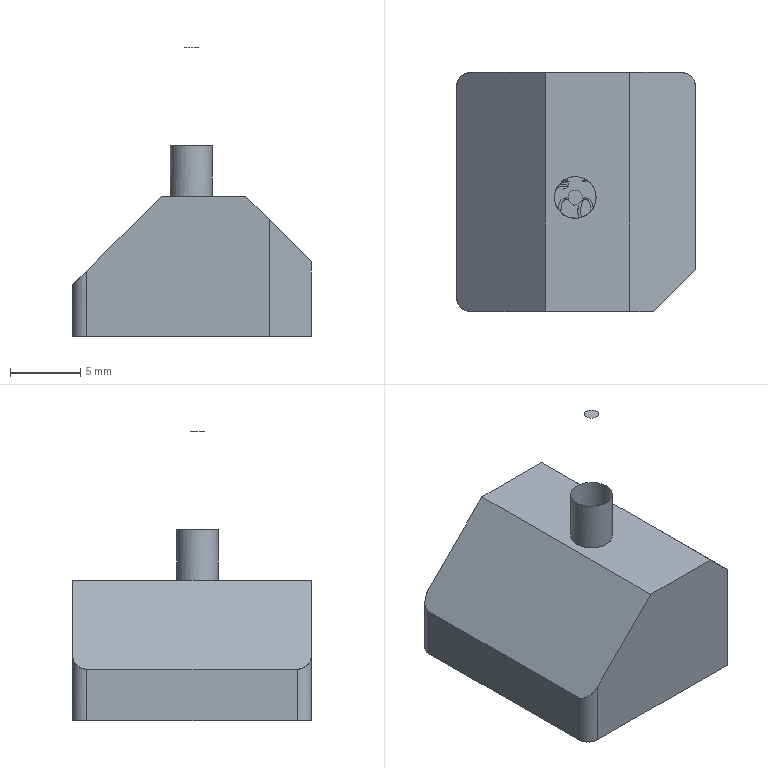NC program | PowerMill | posted with a generic post | part box 17 x 17 x 20.603 mm
Lines 4195 to 5241 of 69435:
N4292 M6
N4293 S18000 M03
N4294 G00 G90 X0.002 Y0.0
N4295 G43 Z10.803 H14
N4296
N4297 G05 P10000 R8
N4298 X0.9692 Y-3.395
N4299 Z0.9255
N4300 G01 Z-0.2745 F1200.0
N4301 X0.9618 Y-3.345 F2000.0
N4302 X0.9504 Y-3.2958
N4303 X0.9351 Y-3.2476
N4304 X0.9161 Y-3.2007
N4305 X0.8935 Y-3.1555
N4306 X0.8674 Y-3.1123
N4307 X0.8379 Y-3.0712
N4308 X0.8053 Y-3.0326
N4309 X0.7698 Y-2.9967
N4310 X0.7315 Y-2.9637
N4311 X0.6907 Y-2.9338
N4312 X0.6478 Y-2.9073
N4313 X0.6028 Y-2.8842
N4314 X0.5562 Y-2.8647
N4315 X0.5082 Y-2.849
N4316 X0.459 Y-2.8371
N4317 X0.4091 Y-2.8291
N4318 X0.3588 Y-2.8251
N4319 X0.3083 Y-2.825
N4320 X0.2634 Y-2.8283
N4321 X0.1652 Y-2.8391
N4322 X0.0665 Y-2.8459
N4323 X-0.0324 Y-2.8486
N4324 X-0.1315 Y-2.8474
N4325 X-0.2305 Y-2.8422
N4326 X-0.3293 Y-2.833
N4327 X-0.4272 Y-2.8199
N4328 X-0.5246 Y-2.8028
N4329 X-0.6211 Y-2.7819
N4330 X-0.7168 Y-2.757
N4331 X-0.8114 Y-2.7283
N4332 X-0.9047 Y-2.6957
N4333 X-0.9966 Y-2.6595
N4334 X-1.0871 Y-2.6195
N4335 X-1.1759 Y-2.5759
N4336 X-1.2629 Y-2.5287
N4337 X-1.3478 Y-2.4781
N4338 X-1.4307 Y-2.4241
N4339 X-1.5112 Y-2.3668
N4340 X-1.5894 Y-2.3063
N4341 X-1.6651 Y-2.2428
N4342 X-1.7381 Y-2.1762
N4343 X-1.8084 Y-2.1067
N4344 X-1.8759 Y-2.0344
N4345 X-1.9404 Y-1.9595
N4346 X-2.0018 Y-1.882
N4347 X-2.06 Y-1.8021
N4348 X-2.115 Y-1.7199
N4349 X-2.1666 Y-1.6355
N4350 X-2.2148 Y-1.5491
N4351 X-2.2594 Y-1.4607
N4352 X-2.3005 Y-1.3706
N4353 X-2.3379 Y-1.2789
N4354 X-2.3716 Y-1.1859
N4355 X-2.4014 Y-1.0915
N4356 X-2.4275 Y-0.9961
N4357 X-2.4496 Y-0.8997
N4358 X-2.4679 Y-0.8025
N4359 X-2.4822 Y-0.7053
N4360 X-2.4925 Y-0.6076
N4361 X-2.4989 Y-0.5095
N4362 X-2.5012 Y-0.4109
N4363 X-2.4996 Y-0.3122
N4364 X-2.4941 Y-0.2135
N4365 X-2.4845 Y-0.1149
N4366 X-2.4709 Y-0.0168
N4367 X-2.4534 Y0.0808
N4368 X-2.432 Y0.1776
N4369 X-2.4066 Y0.2734
N4370 X-2.3775 Y0.368
N4371 X-2.3447 Y0.4612
N4372 X-2.3081 Y0.5529
N4373 X-2.268 Y0.6429
N4374 X-2.224 Y0.7315
N4375 X-2.1766 Y0.8183
N4376 X-2.1257 Y0.9031
N4377 X-2.0713 Y0.9858
N4378 X-2.0137 Y1.0662
N4379 X-1.9529 Y1.1442
N4380 X-1.889 Y1.2197
N4381 X-1.8221 Y1.2926
N4382 X-1.7523 Y1.3626
N4383 X-1.6797 Y1.4298
N4384 X-1.6045 Y1.4941
N4385 X-1.5267 Y1.5552
N4386 X-1.4466 Y1.6131
N4387 X-1.3643 Y1.6677
N4388 X-1.2797 Y1.719
N4389 X-1.1931 Y1.7669
N4390 X-1.1047 Y1.8112
N4391 X-1.0146 Y1.8519
N4392 X-0.9229 Y1.8889
N4393 X-0.8298 Y1.9222
N4394 X-0.7355 Y1.9516
N4395 X-0.6401 Y1.9773
N4396 X-0.5437 Y1.999
N4397 X-0.4465 Y2.0169
N4398 X-0.3488 Y2.0307
N4399 X-0.2501 Y2.0407
N4400 X-0.1512 Y2.0467
N4401 X-0.0523 Y2.0487
N4402 X0.0466 Y2.0467
N4403 X0.1452 Y2.0407
N4404 X0.2434 Y2.0308
N4405 X0.3399 Y2.0171
N4406 X0.4355 Y1.9997
N4407 X0.5307 Y1.9785
N4408 X0.6246 Y1.9534
N4409 X0.7169 Y1.9248
N4410 X0.808 Y1.8926
N4411 X0.8999 Y1.856
N4412 X0.9902 Y1.8157
N4413 X1.0789 Y1.7718
N4414 X1.1656 Y1.7244
N4415 X1.2504 Y1.6735
N4416 X1.3331 Y1.6191
N4417 X1.4135 Y1.5615
N4418 X1.4916 Y1.5007
N4419 X1.5671 Y1.4368
N4420 X1.6399 Y1.3699
N4421 X1.71 Y1.3001
N4422 X1.7772 Y1.2275
N4423 X1.8414 Y1.1523
N4424 X1.9025 Y1.0747
N4425 X1.9604 Y0.9946
N4426 X2.015 Y0.9123
N4427 X2.0663 Y0.8278
N4428 X2.1141 Y0.7413
N4429 X2.1584 Y0.6529
N4430 X2.1991 Y0.5628
N4431 X2.2362 Y0.4711
N4432 X2.2695 Y0.3779
N4433 X2.299 Y0.2835
N4434 X2.3247 Y0.1879
N4435 X2.3465 Y0.0913
N4436 X2.3644 Y-0.006
N4437 X2.3784 Y-0.1038
N4438 X2.3884 Y-0.2021
N4439 X2.3944 Y-0.3007
N4440 X2.3965 Y-0.3994
N4441 X2.3945 Y-0.4982
N4442 X2.3885 Y-0.5968
N4443 X2.3786 Y-0.6951
N4444 X2.3646 Y-0.7929
N4445 X2.3468 Y-0.8902
N4446 X2.325 Y-0.9867
N4447 X2.2993 Y-1.0823
N4448 X2.2698 Y-1.1768
N4449 X2.2365 Y-1.2701
N4450 X2.1994 Y-1.3619
N4451 X2.1587 Y-1.4522
N4452 X2.1144 Y-1.5407
N4453 X2.0666 Y-1.6273
N4454 X2.0153 Y-1.7119
N4455 X1.9607 Y-1.7944
N4456 X1.9029 Y-1.8743
N4457 X1.842 Y-1.9518
N4458 X1.778 Y-2.0268
N4459 X1.7109 Y-2.0992
N4460 X1.6409 Y-2.169
N4461 X1.568 Y-2.2359
N4462 X1.4924 Y-2.2999
N4463 X1.4143 Y-2.3609
N4464 X1.3337 Y-2.4186
N4465 X1.251 Y-2.473
N4466 X1.1662 Y-2.524
N4467 X1.0795 Y-2.5715
N4468 X0.991 Y-2.6154
N4469 X0.901 Y-2.6557
N4470 X0.8094 Y-2.6922
N4471 X0.7165 Y-2.725
N4472 X0.622 Y-2.7542
N4473 X0.5264 Y-2.7795
N4474 X0.4298 Y-2.8009
N4475 X0.3324 Y-2.8184
N4476 X0.2634 Y-2.8283
N4477 X0.2138 Y-2.8375
N4478 X0.165 Y-2.8506
N4479 X0.1173 Y-2.8675
N4480 X0.0712 Y-2.8881
N4481 X0.0268 Y-2.9123
N4482 X-0.0156 Y-2.9399
N4483 X-0.0556 Y-2.9707
N4484 X-0.093 Y-3.0046
N4485 X-0.1277 Y-3.0414
N4486 X-0.1594 Y-3.0808
N4487 X-0.1878 Y-3.1225
N4488 X-0.2129 Y-3.1664
N4489 X-0.2344 Y-3.2121
N4490 X-0.2523 Y-3.2594
N4491 X-0.2663 Y-3.3079
N4492 X-0.2766 Y-3.3574
N4493 X-0.2828 Y-3.4076
N4494 X-0.2851 Y-3.458
N4495 X-0.2834 Y-3.5085
N4496 X-0.2785 Y-3.5532
N4497 X0.9793 Y-3.3881 Z-0.3144
N4498 X0.971 Y-3.3383
N4499 X0.9588 Y-3.2893
N4500 X0.9428 Y-3.2413
N4501 X0.923 Y-3.1948
N4502 X0.8996 Y-3.15
N4503 X0.8727 Y-3.1072
N4504 X0.8426 Y-3.0666
N4505 X0.8093 Y-3.0286
N4506 X0.7732 Y-2.9933
N4507 X0.7344 Y-2.9609
N4508 X0.6931 Y-2.9318
N4509 X0.6497 Y-2.9059
N4510 X0.6044 Y-2.8836
N4511 X0.5574 Y-2.8649
N4512 X0.5091 Y-2.85
N4513 X0.4598 Y-2.8389
N4514 X0.4098 Y-2.8318
N4515 X0.3594 Y-2.8286
N4516 X0.3089 Y-2.8294
N4517 X0.2641 Y-2.8335
N4518 X0.2075 Y-2.8407
N4519 X0.1097 Y-2.849
N4520 X0.0107 Y-2.8535
N4521 X-0.0888 Y-2.854
N4522 X-0.1885 Y-2.8505
N4523 X-0.2877 Y-2.843
N4524 X-0.3857 Y-2.8316
N4525 X-0.4829 Y-2.8164
N4526 X-0.5795 Y-2.7972
N4527 X-0.6754 Y-2.7741
N4528 X-0.7704 Y-2.7471
N4529 X-0.8643 Y-2.7162
N4530 X-0.9571 Y-2.6816
N4531 X-1.0484 Y-2.6432
N4532 X-1.1382 Y-2.6011
N4533 X-1.2263 Y-2.5554
N4534 X-1.3124 Y-2.5063
N4535 X-1.3963 Y-2.4537
N4536 X-1.4781 Y-2.3979
N4537 X-1.5574 Y-2.3389
N4538 X-1.6342 Y-2.2768
N4539 X-1.7083 Y-2.2116
N4540 X-1.78 Y-2.1434
N4541 X-1.8489 Y-2.0723
N4542 X-1.9149 Y-1.9985
N4543 X-1.9778 Y-1.9221
N4544 X-2.0376 Y-1.8432
N4545 X-2.0942 Y-1.762
N4546 X-2.1475 Y-1.6785
N4547 X-2.1974 Y-1.5929
N4548 X-2.2438 Y-1.5053
N4549 X-2.2866 Y-1.4159
N4550 X-2.3258 Y-1.325
N4551 X-2.3612 Y-1.2325
N4552 X-2.3929 Y-1.1387
N4553 X-2.4208 Y-1.0438
N4554 X-2.4449 Y-0.9477
N4555 X-2.465 Y-0.8508
N4556 X-2.4813 Y-0.7532
N4557 X-2.4935 Y-0.655
N4558 X-2.5019 Y-0.5564
N4559 X-2.5062 Y-0.4575
N4560 X-2.5065 Y-0.3586
N4561 X-2.5029 Y-0.2598
N4562 X-2.4952 Y-0.1613
N4563 X-2.4836 Y-0.0631
N4564 X-2.468 Y0.0345
N4565 X-2.4485 Y0.1315
N4566 X-2.4251 Y0.2277
N4567 X-2.3978 Y0.3229
N4568 X-2.3668 Y0.4169
N4569 X-2.3319 Y0.5096
N4570 X-2.2934 Y0.6009
N4571 X-2.2512 Y0.6905
N4572 X-2.2054 Y0.7783
N4573 X-2.1561 Y0.8642
N4574 X-2.1035 Y0.948
N4575 X-2.0475 Y1.0295
N4576 X-1.9883 Y1.1087
N4577 X-1.9259 Y1.1855
N4578 X-1.8605 Y1.2597
N4579 X-1.7922 Y1.3312
N4580 X-1.7209 Y1.4
N4581 X-1.6469 Y1.4659
N4582 X-1.5703 Y1.5287
N4583 X-1.4912 Y1.5884
N4584 X-1.4098 Y1.6449
N4585 X-1.3261 Y1.698
N4586 X-1.2404 Y1.7477
N4587 X-1.1528 Y1.7939
N4588 X-1.0634 Y1.8366
N4589 X-0.9723 Y1.8756
N4590 X-0.8797 Y1.9108
N4591 X-0.7862 Y1.9422
N4592 X-0.6915 Y1.9698
N4593 X-0.5956 Y1.9936
N4594 X-0.4987 Y2.0135
N4595 X-0.4009 Y2.0295
N4596 X-0.3025 Y2.0416
N4597 X-0.2036 Y2.0496
N4598 X-0.1044 Y2.0538
N4599 X-0.0053 Y2.0539
N4600 X0.0938 Y2.05
N4601 X0.1924 Y2.0421
N4602 X0.2906 Y2.0303
N4603 X0.3882 Y2.0145
N4604 X0.4852 Y1.9948
N4605 X0.5814 Y1.9712
N4606 X0.6766 Y1.9437
N4607 X0.7705 Y1.9124
N4608 X0.8629 Y1.8774
N4609 X0.9537 Y1.8388
N4610 X1.043 Y1.7964
N4611 X1.1306 Y1.7505
N4612 X1.2164 Y1.701
N4613 X1.3001 Y1.648
N4614 X1.3818 Y1.5917
N4615 X1.4611 Y1.5321
N4616 X1.5379 Y1.4694
N4617 X1.612 Y1.4038
N4618 X1.6834 Y1.3352
N4619 X1.7519 Y1.2639
N4620 X1.8173 Y1.19
N4621 X1.8797 Y1.1135
N4622 X1.939 Y1.0346
N4623 X1.9953 Y0.9531
N4624 X2.0482 Y0.8694
N4625 X2.0976 Y0.7837
N4626 X2.1436 Y0.6961
N4627 X2.186 Y0.6067
N4628 X2.2247 Y0.5157
N4629 X2.2598 Y0.4231
N4630 X2.2911 Y0.3292
N4631 X2.3186 Y0.234
N4632 X2.3423 Y0.1377
N4633 X2.3621 Y0.0403
N4634 X2.3779 Y-0.0572
N4635 X2.3898 Y-0.1553
N4636 X2.3977 Y-0.2539
N4637 X2.4016 Y-0.3527
N4638 X2.4015 Y-0.4516
N4639 X2.3974 Y-0.5505
N4640 X2.3894 Y-0.649
N4641 X2.3773 Y-0.7472
N4642 X2.3613 Y-0.8448
N4643 X2.3414 Y-0.9418
N4644 X2.3175 Y-1.038
N4645 X2.2898 Y-1.1333
N4646 X2.2584 Y-1.227
N4647 X2.2233 Y-1.3193
N4648 X2.1844 Y-1.4101
N4649 X2.1419 Y-1.4994
N4650 X2.0958 Y-1.587
N4651 X2.0461 Y-1.6728
N4652 X1.993 Y-1.7565
N4653 X1.9365 Y-1.838
N4654 X1.8768 Y-1.9172
N4655 X1.8141 Y-1.9938
N4656 X1.7483 Y-2.0678
N4657 X1.6798 Y-2.1389
N4658 X1.6084 Y-2.2072
N4659 X1.5344 Y-2.2725
N4660 X1.4576 Y-2.335
N4661 X1.3783 Y-2.3943
N4662 X1.2967 Y-2.4504
N4663 X1.2128 Y-2.5032
N4664 X1.1268 Y-2.5525
N4665 X1.0389 Y-2.5984
N4666 X0.9492 Y-2.6407
N4667 X0.8579 Y-2.6793
N4668 X0.7658 Y-2.714
N4669 X0.6723 Y-2.745
N4670 X0.5774 Y-2.7723
N4671 X0.4812 Y-2.7957
N4672 X0.3838 Y-2.8153
N4673 X0.3038 Y-2.8285
N4674 X0.2641 Y-2.8335
N4675 X0.2143 Y-2.8418
N4676 X0.1652 Y-2.854
N4677 X0.1173 Y-2.8701
N4678 X0.0708 Y-2.8899
N4679 X0.026 Y-2.9133
N4680 X-0.0168 Y-2.9401
N4681 X-0.0574 Y-2.9703
N4682 X-0.0954 Y-3.0035
N4683 X-0.1307 Y-3.0397
N4684 X-0.1631 Y-3.0785
N4685 X-0.1923 Y-3.1197
N4686 X-0.2181 Y-3.1631
N4687 X-0.2404 Y-3.2085
N4688 X-0.2591 Y-3.2554
N4689 X-0.274 Y-3.3037
N4690 X-0.2851 Y-3.353
N4691 X-0.2922 Y-3.4031
N4692 X-0.2954 Y-3.4535
N4693 X-0.2946 Y-3.504
N4694 X-0.2905 Y-3.5487
N4695 X0.988 Y-3.3835 Z-0.3543
N4696 X0.979 Y-3.3338
N4697 X0.9661 Y-3.2849
N4698 X0.9493 Y-3.2372
N4699 X0.9289 Y-3.191
N4700 X0.9048 Y-3.1465
N4701 X0.8774 Y-3.1041
N4702 X0.8466 Y-3.064
N4703 X0.8128 Y-3.0264
N4704 X0.7762 Y-2.9916
N4705 X0.7369 Y-2.9599
N4706 X0.6953 Y-2.9313
N4707 X0.6515 Y-2.9061
N4708 X0.6059 Y-2.8844
N4709 X0.5587 Y-2.8664
N4710 X0.5101 Y-2.8521
N4711 X0.4607 Y-2.8418
N4712 X0.4105 Y-2.8353
N4713 X0.3601 Y-2.8329
N4714 X0.3096 Y-2.8344
N4715 X0.2649 Y-2.8391
N4716 X0.243 Y-2.8422
N4717 X0.1448 Y-2.852
N4718 X0.0458 Y-2.8579
N4719 X-0.0537 Y-2.8599
N4720 X-0.1534 Y-2.8578
N4721 X-0.2525 Y-2.8518
N4722 X-0.351 Y-2.8418
N4723 X-0.4486 Y-2.8279
N4724 X-0.546 Y-2.81
N4725 X-0.6425 Y-2.7882
N4726 X-0.7382 Y-2.7626
N4727 X-0.8327 Y-2.7331
N4728 X-0.9259 Y-2.6998
N4729 X-1.0178 Y-2.6627
N4730 X-1.1081 Y-2.622
N4731 X-1.1968 Y-2.5776
N4732 X-1.2837 Y-2.5297
N4733 X-1.3685 Y-2.4783
N4734 X-1.4513 Y-2.4235
N4735 X-1.5317 Y-2.3655
N4736 X-1.6097 Y-2.3043
N4737 X-1.6851 Y-2.2401
N4738 X-1.7578 Y-2.1729
N4739 X-1.8278 Y-2.1028
N4740 X-1.8948 Y-2.03
N4741 X-1.9589 Y-1.9545
N4742 X-2.0198 Y-1.8767
N4743 X-2.0777 Y-1.7962
N4744 X-2.1323 Y-1.7135
N4745 X-2.1836 Y-1.6287
N4746 X-2.2313 Y-1.5419
N4747 X-2.2755 Y-1.4532
N4748 X-2.3161 Y-1.3629
N4749 X-2.353 Y-1.2709
N4750 X-2.3862 Y-1.1775
N4751 X-2.4157 Y-1.0828
N4752 X-2.4413 Y-0.9869
N4753 X-2.463 Y-0.89
N4754 X-2.4808 Y-0.7928
N4755 X-2.4947 Y-0.6949
N4756 X-2.5046 Y-0.5965
N4757 X-2.5105 Y-0.4977
N4758 X-2.5125 Y-0.3988
N4759 X-2.5104 Y-0.2997
N4760 X-2.5044 Y-0.2009
N4761 X-2.4943 Y-0.1023
N4762 X-2.4803 Y-0.0043
N4763 X-2.4624 Y0.0932
N4764 X-2.4406 Y0.1898
N4765 X-2.4149 Y0.2855
N4766 X-2.3854 Y0.3801
N4767 X-2.3521 Y0.4735
N4768 X-2.315 Y0.5654
N4769 X-2.2743 Y0.6558
N4770 X-2.23 Y0.7444
N4771 X-2.1821 Y0.8312
N4772 X-2.1308 Y0.916
N4773 X-2.0761 Y0.9986
N4774 X-2.0182 Y1.0789
N4775 X-1.9571 Y1.1567
N4776 X-1.8929 Y1.2321
N4777 X-1.8258 Y1.3048
N4778 X-1.7557 Y1.3748
N4779 X-1.6828 Y1.442
N4780 X-1.6072 Y1.5062
N4781 X-1.5291 Y1.5674
N4782 X-1.4486 Y1.6254
N4783 X-1.3658 Y1.68
N4784 X-1.2809 Y1.7313
N4785 X-1.1941 Y1.7791
N4786 X-1.1054 Y1.8233
N4787 X-1.015 Y1.8639
N4788 X-0.923 Y1.9009
N4789 X-0.8301 Y1.9339
N4790 X-0.7358 Y1.9632
N4791 X-0.6401 Y1.9888
N4792 X-0.5432 Y2.0105
N4793 X-0.4456 Y2.0283
N4794 X-0.3474 Y2.0422
N4795 X-0.2487 Y2.0521
N4796 X-0.1497 Y2.058
N4797 X-0.0505 Y2.06
N4798 X0.0487 Y2.0579
N4799 X0.1476 Y2.0518
N4800 X0.2462 Y2.0418
N4801 X0.3443 Y2.0278
N4802 X0.4417 Y2.0099
N4803 X0.5386 Y1.988
N4804 X0.6343 Y1.9623
N4805 X0.7287 Y1.9328
N4806 X0.8217 Y1.8996
N4807 X0.9133 Y1.8626
N4808 X1.0034 Y1.8219
N4809 X1.092 Y1.7776
N4810 X1.1789 Y1.7296
N4811 X1.2639 Y1.6781
N4812 X1.3468 Y1.6232
N4813 X1.4273 Y1.5651
N4814 X1.5054 Y1.5038
N4815 X1.5809 Y1.4395
N4816 X1.6536 Y1.3724
N4817 X1.7234 Y1.3025
N4818 X1.7904 Y1.2297
N4819 X1.8544 Y1.1543
N4820 X1.9154 Y1.0763
N4821 X1.9733 Y0.9958
N4822 X2.0279 Y0.913
N4823 X2.0791 Y0.828
N4824 X2.1268 Y0.7411
N4825 X2.171 Y0.6524
N4826 X2.2115 Y0.562
N4827 X2.2484 Y0.4702
N4828 X2.2815 Y0.3769
N4829 X2.3111 Y0.2819
N4830 X2.3367 Y0.1861
N4831 X2.3584 Y0.0896
N4832 X2.3761 Y-0.0072
N4833 X2.3899 Y-0.1049
N4834 X2.3997 Y-0.2034
N4835 X2.4056 Y-0.3025
N4836 X2.4076 Y-0.4019
N4837 X2.4055 Y-0.5012
N4838 X2.3995 Y-0.6003
N4839 X2.3895 Y-0.6987
N4840 X2.3755 Y-0.7964
N4841 X2.3577 Y-0.8931
N4842 X2.3359 Y-0.9896
N4843 X2.3102 Y-1.0853
N4844 X2.2807 Y-1.1799
N4845 X2.2473 Y-1.2733
N4846 X2.2102 Y-1.3653
N4847 X2.1694 Y-1.4558
N4848 X2.125 Y-1.5446
N4849 X2.0771 Y-1.6315
N4850 X2.0257 Y-1.7163
N4851 X1.971 Y-1.799
N4852 X1.9131 Y-1.8793
N4853 X1.8521 Y-1.9571
N4854 X1.788 Y-2.0323
N4855 X1.7209 Y-2.1049
N4856 X1.6511 Y-2.1746
N4857 X1.578 Y-2.242
N4858 X1.5024 Y-2.3063
N4859 X1.4244 Y-2.3674
N4860 X1.3441 Y-2.4252
N4861 X1.2615 Y-2.4798
N4862 X1.1768 Y-2.5309
N4863 X1.0901 Y-2.5786
N4864 X1.0014 Y-2.6229
N4865 X0.9109 Y-2.6635
N4866 X0.8186 Y-2.7006
N4867 X0.7255 Y-2.7338
N4868 X0.6311 Y-2.7632
N4869 X0.5355 Y-2.7888
N4870 X0.4388 Y-2.8105
N4871 X0.3411 Y-2.8284
N4872 X0.3403 Y-2.8285
N4873 X0.2649 Y-2.8391
N4874 X0.2152 Y-2.8482
N4875 X0.1663 Y-2.8611
N4876 X0.1187 Y-2.8778
N4877 X0.0724 Y-2.8983
N4878 X0.028 Y-2.9223
N4879 X-0.0145 Y-2.9498
N4880 X-0.0546 Y-2.9805
N4881 X-0.0922 Y-3.0143
N4882 X-0.127 Y-3.0509
N4883 X-0.1587 Y-3.0902
N4884 X-0.1873 Y-3.1319
N4885 X-0.2125 Y-3.1756
N4886 X-0.2342 Y-3.2213
N4887 X-0.2522 Y-3.2685
N4888 X-0.2665 Y-3.317
N4889 X-0.2768 Y-3.3665
N4890 X-0.2832 Y-3.4166
N4891 X-0.2857 Y-3.4671
N4892 X-0.2842 Y-3.5175
N4893 X-0.2795 Y-3.5622
N4894 X0.974 Y-3.4082 Z-0.3942
N4895 X0.9662 Y-3.3582
N4896 X0.9546 Y-3.309
N4897 X0.9392 Y-3.2609
N4898 X0.92 Y-3.2142
N4899 X0.8971 Y-3.1691
N4900 X0.8708 Y-3.1259
N4901 X0.8411 Y-3.085
N4902 X0.8083 Y-3.0466
N4903 X0.7726 Y-3.0108
N4904 X0.7342 Y-2.978
N4905 X0.6933 Y-2.9483
N4906 X0.6502 Y-2.922
N4907 X0.6052 Y-2.8991
N4908 X0.5585 Y-2.8798
N4909 X0.5103 Y-2.8643
N4910 X0.4612 Y-2.8526
N4911 X0.4112 Y-2.8449
N4912 X0.3609 Y-2.8411
N4913 X0.3104 Y-2.8413
N4914 X0.2655 Y-2.8448
N4915 X0.178 Y-2.8548
N4916 X0.0791 Y-2.8621
N4917 X-0.0202 Y-2.8653
N4918 X-0.1195 Y-2.8646
N4919 X-0.2188 Y-2.8599
N4920 X-0.3178 Y-2.8512
N4921 X-0.4163 Y-2.8386
N4922 X-0.5141 Y-2.822
N4923 X-0.6112 Y-2.8015
N4924 X-0.7073 Y-2.777
N4925 X-0.8024 Y-2.7488
N4926 X-0.8963 Y-2.7167
N4927 X-0.9888 Y-2.6809
N4928 X-1.0798 Y-2.6414
N4929 X-1.1692 Y-2.5982
N4930 X-1.2568 Y-2.5514
N4931 X-1.3424 Y-2.5012
N4932 X-1.426 Y-2.4476
N4933 X-1.5072 Y-2.3906
N4934 X-1.5862 Y-2.3305
N4935 X-1.6626 Y-2.2672
N4936 X-1.7364 Y-2.201
N4937 X-1.8073 Y-2.1319
N4938 X-1.8755 Y-2.0601
N4939 X-1.9406 Y-1.9855
N4940 X-2.0028 Y-1.9084
N4941 X-2.0618 Y-1.8287
N4942 X-2.1177 Y-1.7467
N4943 X-2.1702 Y-1.6624
N4944 X-2.2193 Y-1.576
N4945 X-2.265 Y-1.4877
N4946 X-2.307 Y-1.3976
N4947 X-2.3454 Y-1.306
N4948 X-2.38 Y-1.213
N4949 X-2.4109 Y-1.1187
N4950 X-2.4379 Y-1.0233
N4951 X-2.461 Y-0.9271
N4952 X-2.4803 Y-0.8299
N4953 X-2.4956 Y-0.7319
N4954 X-2.507 Y-0.6334
N4955 X-2.5144 Y-0.5344
N4956 X-2.5178 Y-0.4352
N4957 X-2.5172 Y-0.336
N4958 X-2.5126 Y-0.2368
N4959 X-2.504 Y-0.1379
N4960 X-2.4915 Y-0.0395
N4961 X-2.4751 Y0.058
N4962 X-2.4547 Y0.1547
N4963 X-2.4305 Y0.2508
N4964 X-2.4023 Y0.3461
N4965 X-2.3702 Y0.4404
N4966 X-2.3345 Y0.5332
N4967 X-2.2951 Y0.6243
N4968 X-2.2521 Y0.7137
N4969 X-2.2056 Y0.8013
N4970 X-2.1556 Y0.8868
N4971 X-2.1022 Y0.9703
N4972 X-2.0455 Y1.0515
N4973 X-1.9855 Y1.1304
N4974 X-1.9224 Y1.2069
N4975 X-1.8562 Y1.2808
N4976 X-1.787 Y1.3521
N4977 X-1.7151 Y1.4205
N4978 X-1.6404 Y1.486
N4979 X-1.5631 Y1.5485
N4980 X-1.4834 Y1.6078
N4981 X-1.4014 Y1.6638
N4982 X-1.3173 Y1.7165
N4983 X-1.2311 Y1.7657
N4984 X-1.1431 Y1.8113
N4985 X-1.0533 Y1.8534
N4986 X-0.962 Y1.8918
N4987 X-0.8691 Y1.9265
N4988 X-0.775 Y1.9574
N4989 X-0.6795 Y1.9845
N4990 X-0.583 Y2.0078
N4991 X-0.4855 Y2.0272
N4992 X-0.3875 Y2.0427
N4993 X-0.2888 Y2.0542
N4994 X-0.1898 Y2.0617
N4995 X-0.0905 Y2.0653
N4996 X0.0088 Y2.0648
N4997 X0.108 Y2.0603
N4998 X0.2069 Y2.0519
N4999 X0.3053 Y2.0395
N5000 X0.4032 Y2.0231
N5001 X0.5004 Y2.0028
N5002 X0.5967 Y1.9786
N5003 X0.6919 Y1.9506
N5004 X0.7859 Y1.9187
N5005 X0.8786 Y1.8831
N5006 X0.9697 Y1.8438
N5007 X1.0592 Y1.8008
N5008 X1.147 Y1.7542
N5009 X1.2327 Y1.7042
N5010 X1.3164 Y1.6508
N5011 X1.3978 Y1.594
N5012 X1.4769 Y1.534
N5013 X1.5535 Y1.4709
N5014 X1.6276 Y1.4048
N5015 X1.6986 Y1.336
N5016 X1.7668 Y1.2644
N5017 X1.8321 Y1.1901
N5018 X1.8944 Y1.1131
N5019 X1.9536 Y1.0335
N5020 X2.0096 Y0.9516
N5021 X2.0624 Y0.8674
N5022 X2.1118 Y0.7811
N5023 X2.1576 Y0.6929
N5024 X2.1999 Y0.6029
N5025 X2.2385 Y0.5113
N5026 X2.2733 Y0.4184
N5027 X2.3044 Y0.3242
N5028 X2.3316 Y0.2289
N5029 X2.355 Y0.1327
N5030 X2.3744 Y0.0358
N5031 X2.39 Y-0.0623
N5032 X2.4016 Y-0.1608
N5033 X2.4092 Y-0.2598
N5034 X2.4129 Y-0.359
N5035 X2.4125 Y-0.4583
N5036 X2.4082 Y-0.5574
N5037 X2.3999 Y-0.6563
N5038 X2.3876 Y-0.7548
N5039 X2.3713 Y-0.8528
N5040 X2.3511 Y-0.9499
N5041 X2.327 Y-1.046
N5042 X2.2991 Y-1.1411
N5043 X2.2674 Y-1.2351
N5044 X2.2319 Y-1.3278
N5045 X2.1927 Y-1.419
N5046 X2.1498 Y-1.5086
N5047 X2.1034 Y-1.5964
N5048 X2.0534 Y-1.6823
N5049 X2.0001 Y-1.7661
N5050 X1.9435 Y-1.8476
N5051 X1.8837 Y-1.9267
N5052 X1.8208 Y-2.0032
N5053 X1.755 Y-2.0771
N5054 X1.6862 Y-2.1483
N5055 X1.6143 Y-2.2169
N5056 X1.5398 Y-2.2825
N5057 X1.4627 Y-2.3451
N5058 X1.3831 Y-2.4046
N5059 X1.3011 Y-2.4608
N5060 X1.2171 Y-2.5137
N5061 X1.131 Y-2.5631
N5062 X1.043 Y-2.609
N5063 X0.9532 Y-2.6513
N5064 X0.8618 Y-2.6899
N5065 X0.7692 Y-2.7248
N5066 X0.6752 Y-2.7559
N5067 X0.5799 Y-2.7832
N5068 X0.4835 Y-2.8067
N5069 X0.386 Y-2.8263
N5070 X0.3747 Y-2.8283
N5071 X0.2766 Y-2.8435
N5072 X0.2655 Y-2.8448
N5073 X0.2156 Y-2.8525
N5074 X0.1664 Y-2.8641
N5075 X0.1183 Y-2.8796
N5076 X0.0716 Y-2.8988
N5077 X0.0265 Y-2.9217
N5078 X-0.0167 Y-2.948
N5079 X-0.0576 Y-2.9777
N5080 X-0.096 Y-3.0104
N5081 X-0.1318 Y-3.0461
N5082 X-0.1646 Y-3.0846
N5083 X-0.1943 Y-3.1254
N5084 X-0.2206 Y-3.1685
N5085 X-0.2435 Y-3.2136
N5086 X-0.2628 Y-3.2603
N5087 X-0.2783 Y-3.3084
N5088 X-0.29 Y-3.3576
N5089 X-0.2977 Y-3.4075
N5090 X-0.3015 Y-3.4579
N5091 X-0.3013 Y-3.5084
N5092 X-0.2978 Y-3.5532
N5093 X0.9815 Y-3.4047 Z-0.4341
N5094 X0.9732 Y-3.3548
N5095 X0.961 Y-3.3058
N5096 X0.9449 Y-3.2579
N5097 X0.9251 Y-3.2114
N5098 X0.9017 Y-3.1666
N5099 X0.8749 Y-3.1237
N5100 X0.8447 Y-3.0832
N5101 X0.8115 Y-3.0451
N5102 X0.7753 Y-3.0098
N5103 X0.7365 Y-2.9775
N5104 X0.6952 Y-2.9483
N5105 X0.6518 Y-2.9225
N5106 X0.6065 Y-2.9002
N5107 X0.5596 Y-2.8815
N5108 X0.5112 Y-2.8666
N5109 X0.4619 Y-2.8555
N5110 X0.4119 Y-2.8484
N5111 X0.3615 Y-2.8452
N5112 X0.311 Y-2.846
N5113 X0.2662 Y-2.8501
N5114 X0.2092 Y-2.8573
N5115 X0.1101 Y-2.8658
N5116 X0.0107 Y-2.8704
N5117 X-0.0888 Y-2.8709
N5118 X-0.1882 Y-2.8674
N5119 X-0.2873 Y-2.86
N5120 X-0.3861 Y-2.8485
N5121 X-0.4844 Y-2.8331
N5122 X-0.5819 Y-2.8138
N5123 X-0.6787 Y-2.7906
N5124 X-0.7742 Y-2.7635
N5125 X-0.8682 Y-2.7328
N5126 X-0.9608 Y-2.6983
N5127 X-1.052 Y-2.6601
N5128 X-1.1418 Y-2.6182
N5129 X-1.23 Y-2.5725
N5130 X-1.3166 Y-2.5233
N5131 X-1.4012 Y-2.4706
N5132 X-1.4836 Y-2.4145
N5133 X-1.5637 Y-2.3551
N5134 X-1.6412 Y-2.2927
N5135 X-1.7161 Y-2.2273
N5136 X-1.7875 Y-2.1598
N5137 X-1.8561 Y-2.0894
N5138 X-1.9221 Y-2.016
N5139 X-1.9854 Y-1.9397
N5140 X-2.0457 Y-1.8606
N5141 X-2.1029 Y-1.779
N5142 X-2.1569 Y-1.6951
N5143 X-2.2074 Y-1.6091
N5144 X-2.2545 Y-1.5213
N5145 X-2.2978 Y-1.4319
N5146 X-2.3374 Y-1.3411
N5147 X-2.3732 Y-1.2491
N5148 X-2.4051 Y-1.156
N5149 X-2.4336 Y-1.0608
N5150 X-2.4582 Y-0.9646
N5151 X-2.479 Y-0.8674
N5152 X-2.4958 Y-0.7694
N5153 X-2.5087 Y-0.6709
N5154 X-2.5176 Y-0.5718
N5155 X-2.5225 Y-0.4725
N5156 X-2.5235 Y-0.3731
N5157 X-2.5204 Y-0.2738
N5158 X-2.5133 Y-0.1747
N5159 X-2.5023 Y-0.076
N5160 X-2.4873 Y0.0222
N5161 X-2.4684 Y0.1198
N5162 X-2.4456 Y0.216
N5163 X-2.419 Y0.3113
N5164 X-2.3886 Y0.4056
N5165 X-2.3543 Y0.4988
N5166 X-2.3163 Y0.5906
N5167 X-2.2745 Y0.6809
N5168 X-2.2292 Y0.7696
N5169 X-2.1803 Y0.8564
N5170 X-2.1279 Y0.9411
N5171 X-2.0723 Y1.0236
N5172 X-2.0135 Y1.1037
N5173 X-1.9516 Y1.1812
N5174 X-1.8867 Y1.2561
N5175 X-1.819 Y1.3281
N5176 X-1.7484 Y1.3974
N5177 X-1.6748 Y1.4641
N5178 X-1.5986 Y1.5277
N5179 X-1.5199 Y1.5883
N5180 X-1.4388 Y1.6457
N5181 X-1.3555 Y1.6998
N5182 X-1.27 Y1.7504
N5183 X-1.1825 Y1.7977
N5184 X-1.0933 Y1.8413
N5185 X-1.0024 Y1.8813
N5186 X-0.91 Y1.9177
N5187 X-0.8162 Y1.9502
N5188 X-0.7211 Y1.979
N5189 X-0.625 Y2.0039
N5190 X-0.528 Y2.025
N5191 X-0.4302 Y2.0421
N5192 X-0.3317 Y2.0553
N5193 X-0.2327 Y2.0646
N5194 X-0.1334 Y2.0698
N5195 X-0.034 Y2.0711
N5196 X0.0654 Y2.0684
N5197 X0.1645 Y2.0616
N5198 X0.2633 Y2.0509
N5199 X0.3615 Y2.0363
N5200 X0.4591 Y2.0177
N5201 X0.5559 Y1.9952
N5202 X0.6517 Y1.9688
N5203 X0.7464 Y1.9385
N5204 X0.8398 Y1.9045
N5205 X0.9317 Y1.8668
N5206 X1.0221 Y1.8254
N5207 X1.1107 Y1.7804
N5208 X1.1975 Y1.7318
N5209 X1.2822 Y1.6798
N5210 X1.3648 Y1.6245
N5211 X1.445 Y1.5659
N5212 X1.5229 Y1.5041
N5213 X1.5982 Y1.4392
N5214 X1.6708 Y1.3714
N5215 X1.7403 Y1.301
N5216 X1.807 Y1.2279
N5217 X1.8707 Y1.152
N5218 X1.9314 Y1.0735
N5219 X1.989 Y0.9925
N5220 X2.0434 Y0.9092
N5221 X2.0944 Y0.8237
N5222 X2.1419 Y0.7362
N5223 X2.1859 Y0.6469
N5224 X2.2263 Y0.5559
N5225 X2.2629 Y0.4635
N5226 X2.2958 Y0.3697
N5227 X2.3248 Y0.2749
N5228 X2.35 Y0.179
N5229 X2.3713 Y0.0824
N5230 X2.3887 Y-0.015
N5231 X2.4022 Y-0.1135
N5232 X2.4117 Y-0.2124
N5233 X2.4173 Y-0.3116
N5234 X2.4188 Y-0.411
N5235 X2.4164 Y-0.5102
N5236 X2.41 Y-0.6093
N5237 X2.3996 Y-0.7079
N5238 X2.3852 Y-0.8061
N5239 X2.3669 Y-0.9036
N5240 X2.3446 Y-1.0006
N5241 X2.3185 Y-1.0967
N5242 X2.2885 Y-1.1916
N5243 X2.2547 Y-1.2852
N5244 X2.2173 Y-1.3773
N5245 X2.1761 Y-1.4679
N5246 X2.1314 Y-1.5566
N5247 X2.0838 Y-1.6422
N5248 X2.0323 Y-1.7268
N5249 X1.9771 Y-1.8098
N5250 X1.9184 Y-1.8908
N5251 X1.8566 Y-1.9692
N5252 X1.7922 Y-2.0445
N5253 X1.7255 Y-2.1165
N5254 X1.6565 Y-2.1852
N5255 X1.5833 Y-2.2525
N5256 X1.5074 Y-2.3168
N5257 X1.4289 Y-2.378
N5258 X1.3481 Y-2.436
N5259 X1.265 Y-2.4907
N5260 X1.1798 Y-2.5421
N5261 X1.0926 Y-2.5899
N5262 X1.0035 Y-2.6342
N5263 X0.9128 Y-2.6749
N5264 X0.8205 Y-2.7119
N5265 X0.7269 Y-2.7451
N5266 X0.6321 Y-2.7746
N5267 X0.5363 Y-2.8001
N5268 X0.4396 Y-2.8218
N5269 X0.4059 Y-2.8284
N5270 X0.3078 Y-2.8448
N5271 X0.2662 Y-2.8501
N5272 X0.2164 Y-2.8584
N5273 X0.1673 Y-2.8706
N5274 X0.1194 Y-2.8867
N5275 X0.0729 Y-2.9065
N5276 X0.0281 Y-2.9299
N5277 X-0.0147 Y-2.9568
N5278 X-0.0553 Y-2.9869
N5279 X-0.0933 Y-3.0202
N5280 X-0.1286 Y-3.0563
N5281 X-0.1609 Y-3.0951
N5282 X-0.1901 Y-3.1364
N5283 X-0.2159 Y-3.1798
N5284 X-0.2383 Y-3.2251
N5285 X-0.2569 Y-3.2721
N5286 X-0.2719 Y-3.3204
N5287 X-0.2829 Y-3.3697
N5288 X-0.2901 Y-3.4197
N5289 X-0.2932 Y-3.4701
N5290 X-0.2924 Y-3.5206
N5291 X-0.2883 Y-3.5654
N5292 X0.9887 Y-3.4019 Z-0.474
N5293 X0.9798 Y-3.3522
N5294 X0.967 Y-3.3033
N5295 X0.9504 Y-3.2556
N5296 X0.9301 Y-3.2093
N5297 X0.9062 Y-3.1648
N5298 X0.8788 Y-3.1223
N5299 X0.8482 Y-3.0821
N5300 X0.8145 Y-3.0444
N5301 X0.7779 Y-3.0095
N5302 X0.7387 Y-2.9777
N5303 X0.6971 Y-2.949
N5304 X0.6534 Y-2.9237
N5305 X0.6078 Y-2.9019
N5306 X0.5607 Y-2.8837
N5307 X0.5122 Y-2.8694
N5308 X0.4628 Y-2.8589
N5309 X0.4127 Y-2.8523
N5310 X0.3622 Y-2.8497
N5311 X0.3117 Y-2.8512
N5312 X0.267 Y-2.8558
N5313 X0.2395 Y-2.8596
N5314 X0.1405 Y-2.8692
N5315 X0.041 Y-2.875
N5316 X-0.059 Y-2.8767
N5317 X-0.1587 Y-2.8745
N5318 X-0.258 Y-2.8682
N5319 X-0.3567 Y-2.8581
N5320 X-0.4547 Y-2.8439
N5321 X-0.552 Y-2.8259
N5322 X-0.649 Y-2.8039
N5323 X-0.7451 Y-2.778
N5324 X-0.84 Y-2.7483
N5325 X-0.9336 Y-2.7148
N5326 X-1.0258 Y-2.6776
N5327 X-1.1163 Y-2.6368
N5328 X-1.2052 Y-2.5923
N5329 X-1.2922 Y-2.5443
N5330 X-1.3772 Y-2.4928
N5331 X-1.46 Y-2.4379
N5332 X-1.5406 Y-2.3798
N5333 X-1.6188 Y-2.3185
N5334 X-1.6946 Y-2.254
N5335 X-1.7677 Y-2.1866
N5336 X-1.8379 Y-2.1165
N5337 X-1.9054 Y-2.0435
N5338 X-1.9698 Y-1.9678